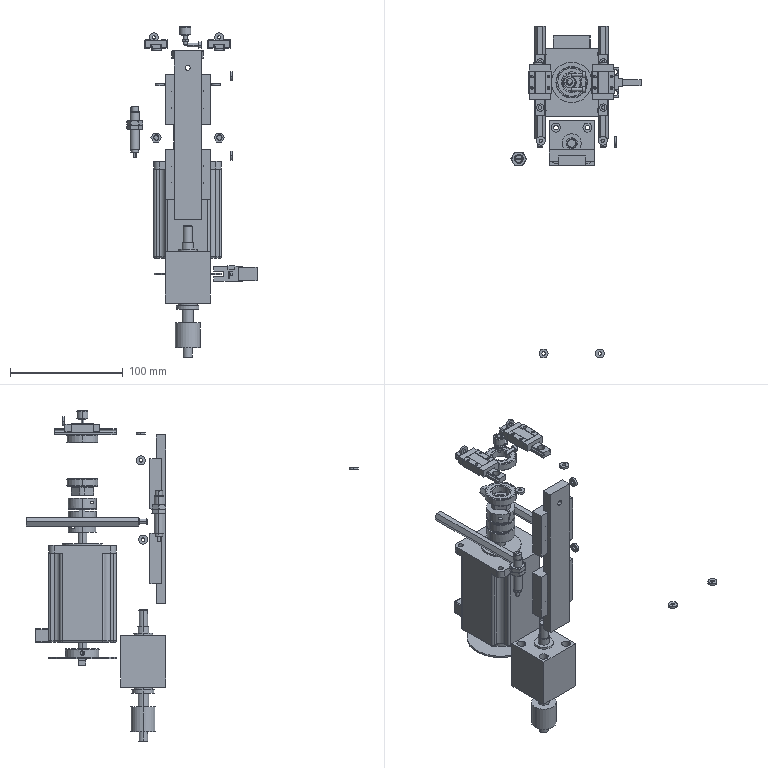Part | NX | 30 solids | 1381 faces | box 115.528 x 294.9 x 294.4 mm | volume 482221 mm3 | plane 904 | cylinder 323 | cone 108 | torus 40 | sphere 4 | spline 2 | commonest cylinder face diameters 8 x56 2.5 x38 2 x24 3 x22 3.2 x16 10 x16